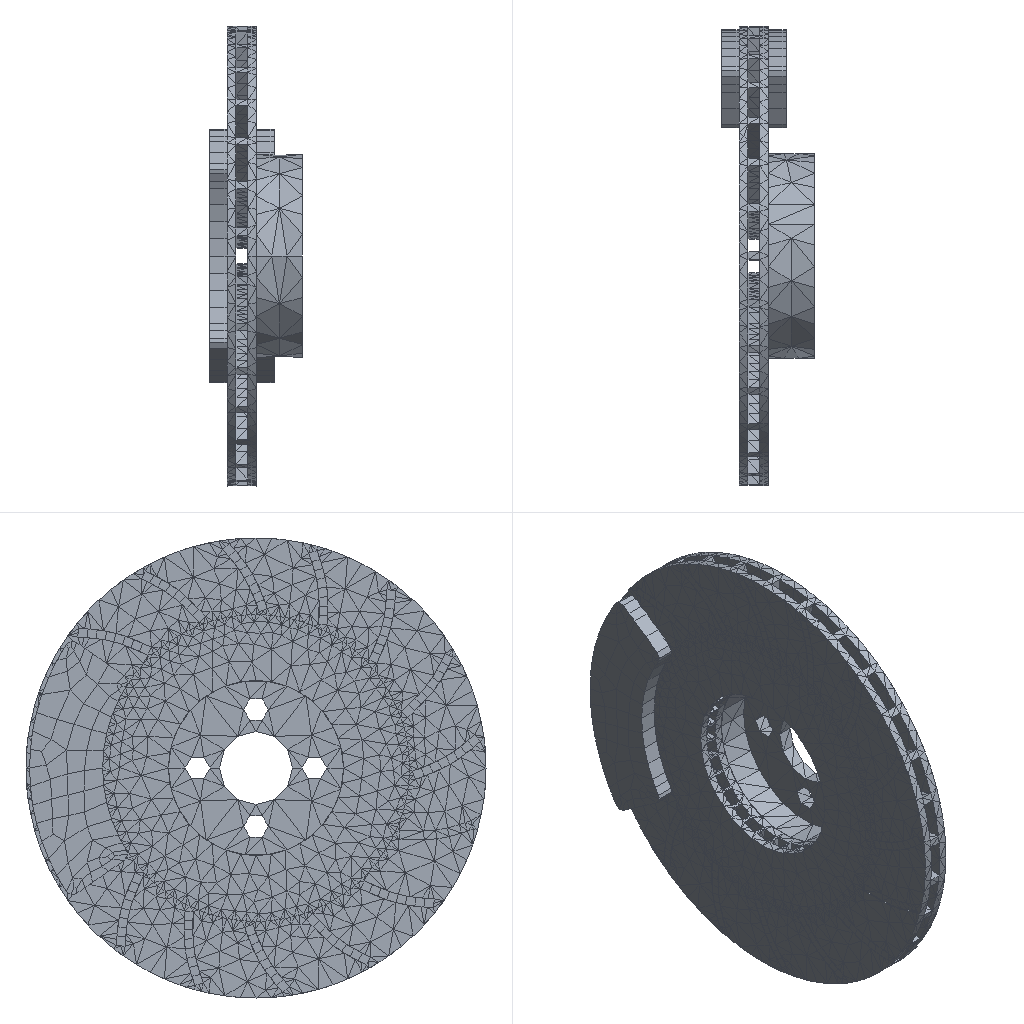Simulation study | ansys workbench
Ansys APDL input file, long lists of numbers shortened:
/batch
/config,noeldb,1     ! force off writing results to database
*get,_wallstrt,active,,time,wall
! ANSYS input file written by Workbench version 2022 R1
! File used for geometry attach:
/title,1111--____ (C5)
! ****** Begin Custom Load Command Snippet ******
/COM, ACT Extensions:
/COM,     LSDYNA, 2021.1
/COM,
! ****** End   Custom Load Command Snippet ******
*DIM,_wb_ProjectScratch_dir,string,248
_wb_ProjectScratch_dir(1) = ''
*DIM,_wb_SolverFiles_dir,string,248
_wb_SolverFiles_dir(1) = ''
*DIM,_wb_userfiles_dir,string,248
_wb_userfiles_dir(1) = ''
/com,--- Data in consistent NMM units. See Solving Units in the help system for more information.
/units,MPA
/nopr
/wb,file,start              !  signify a WB generated input file
/prep7
! Turn off shape checking because checks already performed inside WB mesher.
! See help system for more information.
SHPP,OFF,,NOWARN
/nolist
etcon,set             ! allow ANSYS to choose best KEYOP's for 180x elements, resets any applicable keyopt to MAPDL defaults
/com,*********** Nodes for the whole assembly ***********
nblock,3,,31611
(1i9,3e20.9e3)
        1    -5.687067418E+00     4.219548714E+00     4.362788327E+02
! (28737 more lines like these left out)
-1
/wb,elem,start            !  set before creation of elements
/com,*********** Elements for Body 1 "model|____-____/____1" ***********
et,1,186
keyo,1,2,1          ! set full integration on SOLID186
eblock,19,solid,,71
(19i9)
        1        1        1        1        0        0        0        0       20        0      113     1461     1475     1498     1507     1554     1540     1517     1508
! (141 more lines like these left out)
-1
/com,*********** Elements for Body 2 "model|____-____/____1[2]" ***********
et,2,186
keyo,2,2,1          ! set full integration on SOLID186
eblock,19,solid,,75
(19i9)
        2        2        2        2        0        0        0        0       20        0      184     2069     2116     2084     2070     2164     2117     2149     2163
! (149 more lines like these left out)
-1
/com,*********** Elements for Body 3 "model|____-____3[1]" ***********
et,3,187
eblock,19,solid,,12722
(19i9)
        3        3        3        3        0        0        0        0       10        0      763     6344     7992     7917     7984    24419    28694    24417    24418
! (25443 more lines like these left out)
-1
/com,*********** Elements for Body 4 "model|____-____3[2]" ***********
et,4,187
eblock,19,solid,,496
(19i9)
        4        4        4        4        0        0        0        0       10        0      267     2871     3008     2982     3017     3464     3916     3463     3465
! (991 more lines like these left out)
-1
/com,*********** Elements for Body 5 "model|Solid" ***********
et,5,186
keyo,5,2,1          ! set full integration on SOLID186
eblock,19,solid,,8
(19i9)
        5        5        5        5        0        0        0        0       20        0       33      417      426      425      424      452      437      444      445
! (15 more lines like these left out)
-1
! (14 more sections like these left out)
/wb,elem,end               !  done creating elements
/com,*********** Send User Defined Coordinate System(s) ***********
csys,0
toffst,273.15,  ! Temperature offset from absolute zero
/com,*********** Set Reference Temperature ***********
tref,22.
/wb,mat,start              !  starting to send materials
/com,*********** Send Materials ***********
Temperature = 'TEMP' ! Temperature
MP,DENS,1,7.85e-09,	! tonne mm^-3
MP,ALPX,1,1.2e-05,	! C^-1
MP,C,1,434000000,	! mm^2 s^-2 C^-1
MP,KXX,1,60.5,	! tonne mm s^-3 C^-1
MP,RSVX,1,0.00017,	! ohm mm
MP,EX,1,200000,	! tonne s^-2 mm^-1
MP,NUXY,1,0.3,
MP,MURX,1,10000,
Temperature = 'TEMP' ! Temperature
MP,DENS,2,7.85e-09,	! tonne mm^-3
MP,ALPX,2,1.2e-05,	! C^-1
MP,C,2,434000000,	! mm^2 s^-2 C^-1
MP,KXX,2,60.5,	! tonne mm s^-3 C^-1
MP,RSVX,2,0.00017,	! ohm mm
MP,EX,2,200000,	! tonne s^-2 mm^-1
MP,NUXY,2,0.3,
MP,MURX,2,10000,
Temperature = 'TEMP' ! Temperature
MP,DENS,3,7.85e-09,	! tonne mm^-3
MP,ALPX,3,1.2e-05,	! C^-1
MP,C,3,434000000,	! mm^2 s^-2 C^-1
MP,KXX,3,60.5,	! tonne mm s^-3 C^-1
MP,RSVX,3,0.00017,	! ohm mm
MP,EX,3,200000,	! tonne s^-2 mm^-1
MP,NUXY,3,0.3,
MP,MURX,3,10000,
Temperature = 'TEMP' ! Temperature
MP,DENS,4,7.85e-09,	! tonne mm^-3
MP,ALPX,4,1.2e-05,	! C^-1
MP,C,4,434000000,	! mm^2 s^-2 C^-1
MP,KXX,4,60.5,	! tonne mm s^-3 C^-1
MP,RSVX,4,0.00017,	! ohm mm
MP,EX,4,200000,	! tonne s^-2 mm^-1
MP,NUXY,4,0.3,
MP,MURX,4,10000,
Temperature = 'TEMP' ! Temperature
MP,DENS,5,7.85e-09,	! tonne mm^-3
MP,ALPX,5,1.2e-05,	! C^-1
MP,C,5,434000000,	! mm^2 s^-2 C^-1
MP,KXX,5,60.5,	! tonne mm s^-3 C^-1
MP,RSVX,5,0.00017,	! ohm mm
MP,EX,5,200000,	! tonne s^-2 mm^-1
MP,NUXY,5,0.3,
MP,MURX,5,10000,
Temperature = 'TEMP' ! Temperature
MP,DENS,6,7.85e-09,	! tonne mm^-3
MP,ALPX,6,1.2e-05,	! C^-1
MP,C,6,434000000,	! mm^2 s^-2 C^-1
MP,KXX,6,60.5,	! tonne mm s^-3 C^-1
MP,RSVX,6,0.00017,	! ohm mm
MP,EX,6,200000,	! tonne s^-2 mm^-1
MP,NUXY,6,0.3,
MP,MURX,6,10000,
Temperature = 'TEMP' ! Temperature
MP,DENS,7,7.85e-09,	! tonne mm^-3
MP,ALPX,7,1.2e-05,	! C^-1
MP,C,7,434000000,	! mm^2 s^-2 C^-1
MP,KXX,7,60.5,	! tonne mm s^-3 C^-1
MP,RSVX,7,0.00017,	! ohm mm
MP,EX,7,200000,	! tonne s^-2 mm^-1
MP,NUXY,7,0.3,
MP,MURX,7,10000,
Temperature = 'TEMP' ! Temperature
MP,DENS,8,7.85e-09,	! tonne mm^-3
MP,ALPX,8,1.2e-05,	! C^-1
MP,C,8,434000000,	! mm^2 s^-2 C^-1
MP,KXX,8,60.5,	! tonne mm s^-3 C^-1
MP,RSVX,8,0.00017,	! ohm mm
MP,EX,8,200000,	! tonne s^-2 mm^-1
MP,NUXY,8,0.3,
MP,MURX,8,10000,
Temperature = 'TEMP' ! Temperature
MP,DENS,9,7.85e-09,	! tonne mm^-3
MP,ALPX,9,1.2e-05,	! C^-1
MP,C,9,434000000,	! mm^2 s^-2 C^-1
MP,KXX,9,60.5,	! tonne mm s^-3 C^-1
MP,RSVX,9,0.00017,	! ohm mm
MP,EX,9,200000,	! tonne s^-2 mm^-1
! (92 more lines like these left out)
/wb,mat,end                !  done sending materials
!************************* Model Summary ********************
!model|____-____/____1,	结构钢,	matid,	1
!model|____-____/____1[2],	结构钢,	matid,	2
!model|____-____3[1],	结构钢,	matid,	3
!model|____-____3[2],	结构钢,	matid,	4
!model|Solid,	结构钢,	matid,	5
!model|Solid[2],	结构钢,	matid,	6
!model|Solid[3],	结构钢,	matid,	7
!model|Solid[4],	结构钢,	matid,	8
!model|Solid[5],	结构钢,	matid,	9
!model|Solid[6],	结构钢,	matid,	10
!model|Solid[7],	结构钢,	matid,	11
!model|Solid[8],	结构钢,	matid,	12
!model|Solid[9],	结构钢,	matid,	13
!model|Solid[10],	结构钢,	matid,	14
!model|Solid[11],	结构钢,	matid,	15
!model|Solid[12],	结构钢,	matid,	16
!model|Solid[13],	结构钢,	matid,	17
!model|Solid[14],	结构钢,	matid,	18
!model|Solid[15],	结构钢,	matid,	19
!************************* End Model Summary ********************
! get the diagonal of the bounding box. Needed later for other things
*get,_xmin,node,,mnloc,x
*get,_ymin,node,,mnloc,y
*get,_zmin,node,,mnloc,z
*get,_xmax,node,,mxloc,x
*get,_ymax,node,,mxloc,y
*get,_zmax,node,,mxloc,z
_ASMDIAG=(_xmax-_xmin)*(_xmax-_xmin)+(_ymax-_ymin)*(_ymax-_ymin)+(_zmax-_zmin)*(_zmax-_zmin)
_ASMDIAG=SQRT(_ASMDIAG)
/wb,contact,start          !  starting to send contact
/com,*********** Create Contact "接触区域" ***********
/com,            Real Constant Set For Above Contact Is 21 & 20
*set,tid,21
*set,cid,20
r,tid
r,cid
et,tid,170
et,cid,174
eblock,10,,,71
(15i9)
    22751       21       21       21        0     1554     1540     1517     1508     1908     1847     1815     1817
! (70 more lines like these left out)
-1
eblock,10,,,71
(15i9)
    22822       20       20       20        0     1554     1540     1517     1508     1908     1847     1815     1817
! (70 more lines like these left out)
-1
eblock,10,,,315
(15i9)
    22893       20       21       20        0     4246     7172     4247     4247     9933     9941     4247     9930
! (314 more lines like these left out)
-1
eblock,10,,,315
(15i9)
    23208       21       20       21        0     4246     7172     4247     4247     9933     9941     4247     9930
! (314 more lines like these left out)
-1
keyo,cid,8,2               ! auto create asymmetric contact (from Program Controlled setting)
keyo,cid,10,0              ! adjust contact stiffness each NR iteration (from Program Controlled setting)
keyo,cid,12,5              ! bonded always
keyo,cid,18,1              ! small sliding turned on by application
keyo,cid,2,0               ! augmented Lagrange (from Program Controlled setting)
keyo,cid,4,0               ! on Gauss point (from Program Controlled setting)
keyo,cid,9,1               ! ignore initial gaps/penetration
keyo,cid,7,0               ! No Prediction
rmod,tid,3,10.      ! FKN
rmod,tid,5,0.       ! ICONT
rmod,tid,6,0.       ! PINB
rmod,tid,10,0.      ! CNOF
rmod,tid,12,0.      ! FKT
rmod,tid,36,80      ! WB DSID
rmod,cid,3,10.      ! FKN
rmod,cid,5,0.       ! ICONT
rmod,cid,6,0.       ! PINB
rmod,cid,10,0.      ! CNOF
rmod,cid,12,0.      ! FKT
rmod,cid,36,80      ! WB DSID
/com,*********** Create Contact "接触区域 2" ***********
/com,            Real Constant Set For Above Contact Is 23 & 22
*set,tid,23
*set,cid,22
r,tid
r,cid
et,tid,170
et,cid,174
eblock,10,,,10
(15i9)
    23523       23       23       23        0     1512     1544     1542     1539     1831     1910     1904     1830
! (9 more lines like these left out)
-1
eblock,10,,,10
(15i9)
    23533       22       22       22        0     1512     1544     1542     1539     1831     1910     1904     1830
! (9 more lines like these left out)
-1
eblock,10,,,8
(15i9)
    23543       22       23       22        0      649      653      652      651      718      721      720      717
! (7 more lines like these left out)
-1
eblock,10,,,8
(15i9)
    23551       23       22       23        0      649      653      652      651      718      721      720      717
! (7 more lines like these left out)
-1
keyo,cid,8,2               ! auto create asymmetric contact (from Program Controlled setting)
keyo,cid,10,0              ! adjust contact stiffness each NR iteration (from Program Controlled setting)
keyo,cid,12,5              ! bonded always
keyo,cid,18,1              ! small sliding turned on by application
keyo,cid,2,0               ! augmented Lagrange (from Program Controlled setting)
keyo,cid,4,0               ! on Gauss point (from Program Controlled setting)
keyo,cid,9,1               ! ignore initial gaps/penetration
keyo,cid,7,0               ! No Prediction
rmod,tid,3,10.      ! FKN
rmod,tid,5,0.       ! ICONT
rmod,tid,6,0.       ! PINB
rmod,tid,10,0.      ! CNOF
rmod,tid,12,0.      ! FKT
rmod,tid,36,83      ! WB DSID
rmod,cid,3,10.      ! FKN
rmod,cid,5,0.       ! ICONT
rmod,cid,6,0.       ! PINB
rmod,cid,10,0.      ! CNOF
rmod,cid,12,0.      ! FKT
rmod,cid,36,83      ! WB DSID
/com,*********** Create Contact "接触区域 3" ***********
/com,            Real Constant Set For Above Contact Is 25 & 24
*set,tid,25
*set,cid,24
r,tid
r,cid
et,tid,170
et,cid,174
eblock,10,,,11
(15i9)
    23559       25       25       25        0     1529     1530     1531     1532     1881     1884     1887     1882
! (10 more lines like these left out)
-1
eblock,10,,,11
(15i9)
    23570       24       24       24        0     1529     1530     1531     1532     1881     1884     1887     1882
! (10 more lines like these left out)
-1
eblock,10,,,8
(15i9)
    23581       24       25       24        0      972      957      964      965     1021     1020     1033     1034
! (7 more lines like these left out)
-1
eblock,10,,,8
(15i9)
    23589       25       24       25        0      972      957      964      965     1021     1020     1033     1034
! (7 more lines like these left out)
-1
keyo,cid,8,2               ! auto create asymmetric contact (from Program Controlled setting)
keyo,cid,10,0              ! adjust contact stiffness each NR iteration (from Program Controlled setting)
keyo,cid,12,5              ! bonded always
keyo,cid,18,1              ! small sliding turned on by application
keyo,cid,2,0               ! augmented Lagrange (from Program Controlled setting)
keyo,cid,4,0               ! on Gauss point (from Program Controlled setting)
keyo,cid,9,1               ! ignore initial gaps/penetration
keyo,cid,7,0               ! No Prediction
rmod,tid,3,10.      ! FKN
rmod,tid,5,0.       ! ICONT
rmod,tid,6,0.       ! PINB
rmod,tid,10,0.      ! CNOF
rmod,tid,12,0.      ! FKT
rmod,tid,36,86      ! WB DSID
rmod,cid,3,10.      ! FKN
rmod,cid,5,0.       ! ICONT
rmod,cid,6,0.       ! PINB
rmod,cid,10,0.      ! CNOF
rmod,cid,12,0.      ! FKT
rmod,cid,36,86      ! WB DSID
/com,*********** Create Contact "接触区域 4" ***********
/com,            Real Constant Set For Above Contact Is 27 & 26
*set,tid,27
*set,cid,26
r,tid
r,cid
et,tid,170
et,cid,174
eblock,10,,,14
(15i9)
    23597       27       27       27        0     1554     1540     1517     1508     1908     1847     1815     1817
! (13 more lines like these left out)
-1
eblock,10,,,14
(15i9)
    23611       26       26       26        0     1554     1540     1517     1508     1908     1847     1815     1817
! (13 more lines like these left out)
-1
eblock,10,,,8
(15i9)
    23625       26       27       26        0      337      341      340      339      406      409      408      405
! (7 more lines like these left out)
-1
eblock,10,,,8
(15i9)
    23633       27       26       27        0      337      341      340      339      406      409      408      405
! (7 more lines like these left out)
-1
keyo,cid,8,2               ! auto create asymmetric contact (from Program Controlled setting)
keyo,cid,10,0              ! adjust contact stiffness each NR iteration (from Program Controlled setting)
keyo,cid,12,5              ! bonded always
keyo,cid,18,1              ! small sliding turned on by application
keyo,cid,2,0               ! augmented Lagrange (from Program Controlled setting)
keyo,cid,4,0               ! on Gauss point (from Program Controlled setting)
keyo,cid,9,1               ! ignore initial gaps/penetration
keyo,cid,7,0               ! No Prediction
rmod,tid,3,10.      ! FKN
rmod,tid,5,0.       ! ICONT
rmod,tid,6,0.       ! PINB
rmod,tid,10,0.      ! CNOF
rmod,tid,12,0.      ! FKT
rmod,tid,36,89      ! WB DSID
rmod,cid,3,10.      ! FKN
rmod,cid,5,0.       ! ICONT
rmod,cid,6,0.       ! PINB
rmod,cid,10,0.      ! CNOF
rmod,cid,12,0.      ! FKT
rmod,cid,36,89      ! WB DSID
/com,*********** Create Contact "接触区域 5" ***********
/com,            Real Constant Set For Above Contact Is 29 & 28
*set,tid,29
*set,cid,28
r,tid
r,cid
et,tid,170
et,cid,174
eblock,10,,,75
(15i9)
    23641       29       29       29        0     2149     2163     2164     2117     2531     2556     2443     2442
! (74 more lines like these left out)
-1
eblock,10,,,75
(15i9)
    23716       28       28       28        0     2149     2163     2164     2117     2531     2556     2443     2442
! (74 more lines like these left out)
-1
eblock,10,,,315
(15i9)
    23791       28       29       28        0     7277     7307     7294     7294    27401    27483     7294    27400
! (314 more lines like these left out)
-1
eblock,10,,,315
(15i9)
    24106       29       28       29        0     7277     7307     7294     7294    27401    27483     7294    27400
! (314 more lines like these left out)
-1
keyo,cid,8,2               ! auto create asymmetric contact (from Program Controlled setting)
keyo,cid,10,0              ! adjust contact stiffness each NR iteration (from Program Controlled setting)
keyo,cid,12,5              ! bonded always
keyo,cid,18,1              ! small sliding turned on by application
keyo,cid,2,0               ! augmented Lagrange (from Program Controlled setting)
keyo,cid,4,0               ! on Gauss point (from Program Controlled setting)
keyo,cid,9,1               ! ignore initial gaps/penetration
keyo,cid,7,0               ! No Prediction
rmod,tid,3,10.      ! FKN
rmod,tid,5,0.       ! ICONT
rmod,tid,6,0.       ! PINB
rmod,tid,10,0.      ! CNOF
rmod,tid,12,0.      ! FKT
rmod,tid,36,92      ! WB DSID
rmod,cid,3,10.      ! FKN
rmod,cid,5,0.       ! ICONT
rmod,cid,6,0.       ! PINB
rmod,cid,10,0.      ! CNOF
rmod,cid,12,0.      ! FKT
rmod,cid,36,92      ! WB DSID
! (16 more sections like these left out)
/wb,contact,end            !  done creating contacts
/golist
/wb,load,start             !  starting to send loads
/com,*********** Fixed Supports ***********
CMBLOCK,_FIXEDSU,NODE,      216
(8i10)
      2799      2800      2801      2802      2803      2804      2805      2806
! (26 more lines like these left out)
cmsel,s,_FIXEDSU
d,all,all
nsel,all
/gst,on,on
fini
*get,_numnode,node,0,count
*get,_numelem,elem,0,count
*get, _MAXELEMNUM, elem, 0, NUM, MAX
*get, _MAXNODENUM, node, 0, NUM, MAX
*get, _MAXELEMTYPE, etyp, 0, NUM, MAX
*get, _MAXREALCONST, real, 0, NUM, MAX
/go
/wb,load,end               !  done creating loads
/com,--- Number of total nodes = %_numnode%
/com,--- Number of contact elements = 4296
/com,--- Number of spring elements = 0
/com,--- Number of bearing elements = 0
/com,--- Number of solid elements = 13484
/com,--- Number of condensed parts = 0
/com,--- Number of total elements = %_numelem%
*get,_wallbsol,active,,time,wall
/com,****************************************************************************
/com,*************************    SOLUTION       ********************************
/com,****************************************************************************
/solu
antype,0                   ! static analysis
_thickRatio=  0     ! Ratio of thick parts in the model
eqsl,sparse,,,,,1
cntr,print,1               ! print out contact info and also make no initial contact an error
dmpoption,emat,no             ! Don't combine emat file for DANSYS
dmpoption,esav,no             ! Don't combine esav file for DANSYS
nldiag,cont,iter           ! print out contact info each equilibrium iteration
rescontrol,,none                 ! Do not keep any restart files
/com,****************************************************
/com,******************* SOLVE FOR LS 1 OF 1 ****************
/nopr
/com,*********** Create Imported Load "________" ***********
/nopr
bfblock,2,temp,28738,28738,0
(i9,e20.9e3)
        1     1.672503052e+02
! (28737 more lines like these left out)
bf,end,loc,-1,
/gopr
/gopr
nsub,1,1,1
time,1.
outres,erase
outres,all,none
outres,nsol,all,
outres,rsol,all
outres,eangl,all
outres,etmp,all
outres,veng,all
outres,strs,all,
outres,epel,all,
outres,eppl,all,
outres,epth,all,
outres,cont,all,
! *********** WB SOLVE COMMAND ***********
! check interactive state
*get,ANSINTER_,active,,int
*if,ANSINTER_,ne,0,then
/eof
*endif
solve
/com *************** Write FE CONNECTORS *********
CEWRITE,file,ce,,INTE
/com,****************************************************
/com,*************** FINISHED SOLVE FOR LS 1 *************
*get,_wallasol,active,,time,wall
/nopr
*get,_numnode,node,0,count
*get,_numelem,elem,0,count
*get, _MAXELEMNUM, elem, 0, NUM, MAX
*get, _MAXNODENUM, node, 0, NUM, MAX,,,INTERNAL
*get, _MAXELEMTYPE, etyp, 0, NUM, MAX
*get, _MAXREALCONST, real, 0, NUM, MAX
/gopr
/post1
xmlo,ENCODING,ISO-8859-1
xmlo,parm
/xml,parm,xml
fini
/gopr
*get,_walldone,active,,time,wall
_preptime=(_wallbsol-_wallstrt)*3600
_solvtime=(_wallasol-_wallbsol)*3600
_posttime=(_walldone-_wallasol)*3600
_totaltim=(_walldone-_wallstrt)*3600
*get,_dlbratio,active,0,solu,dlbr
*get,_combtime,active,0,solu,comb
*get,_ssmode,active,0,solu,ssmm
*get,_ndofs,active,0,solu,ndof
*get,_sol_end_time,active,0,set,time
*if,_sol_end_time,eq,1.,then
/fclean				!clean distributed files
*endif
/com,--- Total number of nodes = %_numnode%
/com,--- Total number of elements = %_numelem%
/com,--- Element load balance ratio = %_dlbratio%
/com,--- Time to combine distributed files = %_combtime%
/com,--- Sparse memory mode = %_ssmode%
/com,--- Number of DOF = %_ndofs%
/wb,file,end               ! done with WB generated input